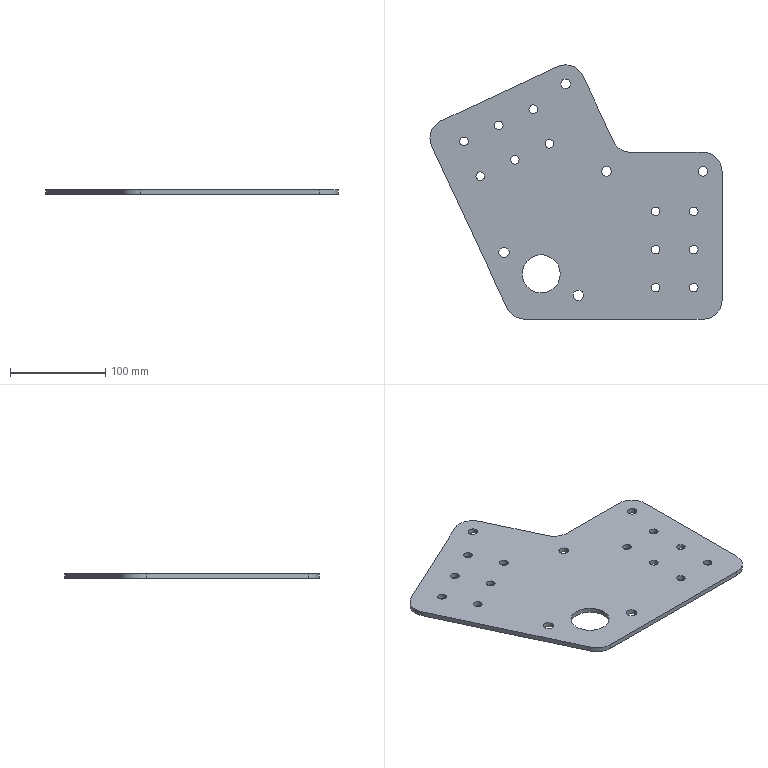Part | STEP file | Ga bi suong | 1 solid | 50 faces | box 306.397 x 266.767 x 5 mm | volume 273503 mm3 | cylinder 42 | plane 8 | commonest cylinder face diameters 9 x24 40 x8 10 x6 11 x4